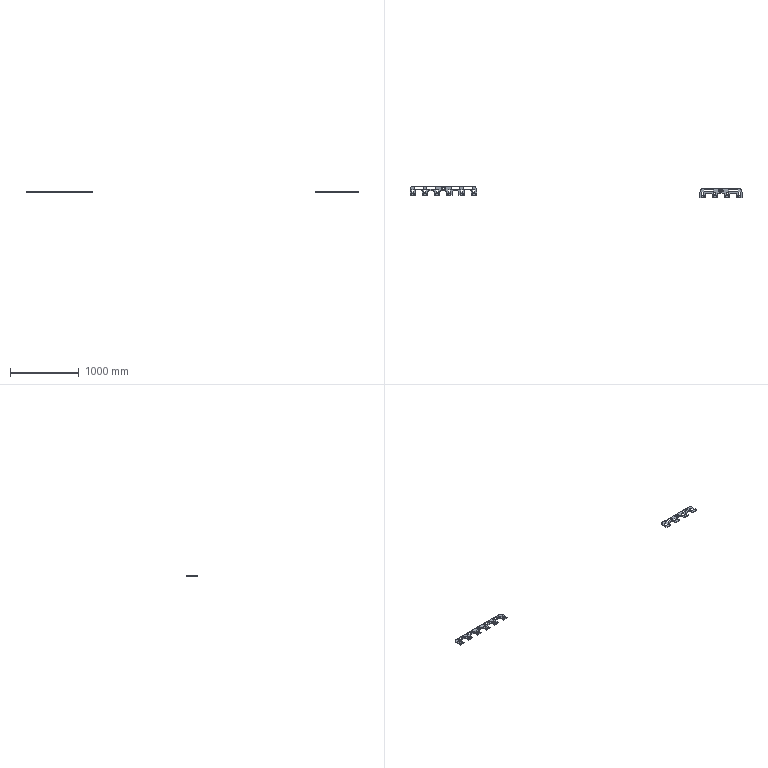NC program | NX | posted with a generic post | part box 4825 x 168.213 x 13 mm
Lines 1 to 137 of 14244:
N10 G17 G21 G94 G90
(FLOOR_WALL_COPY , TOOL : D63)
N12 T01 M6
N14 G54
N16 G17 G0 G90 X-36.5 Y68.997 S6500 M3
N18 G43 Z30. H1
N20 Z4.
N22 G94 G1 Z1. F1500.
N24 X-33.5
N26 X1000.3
N28 Y40.798
N30 X-33.5
N32 Y12.599
N34 X1000.3
N36 Y-15.601
N38 X-33.5
N40 Y-43.8
N42 X1000.3
N44 X1003.3
N46 Z4.
N48 G0 Z30.
N50 X-36.5 Y68.997
N52 Z3.
N54 G1 Z0.
N56 X-33.5
N58 X1000.3
N60 Y40.798
N62 X-33.5
N64 Y12.599
N66 X1000.3
N68 Y-15.601
N70 X-33.5
N72 Y-43.8
N74 X1000.3
N76 X1003.3
N78 Z3.
N80 G0 Z30.
N82 M5
(DRILLING_COPY_1 , TOOL : D6A45)
N84 T07 M6
N86 G54
N88 G17 G0 G90 X947.9 Y-61.2 S5000 M3
N90 G43 Z30. H7
N92 G94 G81 G98 Z-1. F250. R3.
N94 Y-39.2
N96 X907.9
N98 Y-61.2
N100 X770.1 Y-39.2
N102 Y-61.2
N104 X730.1
N106 Y-39.2
N108 X592.3
N110 Y-61.2
N112 X552.3
N114 Y-39.2
N116 X494.115 Y7.131
N118 X509.269 Y22.285
N120 Y43.715
N122 X494.115 Y58.869
N124 X472.685
N126 X457.531 Y43.715
N128 Y22.285
N130 X483.4 Y33.
N132 X472.685 Y7.131
N134 X414.5 Y-39.2
N136 Y-61.2
N138 X374.5
N140 Y-39.2
N142 X236.7
N144 Y-61.2
N146 X196.7
N148 Y-39.2
N150 X58.9
N152 Y-61.2
N154 X18.9
N156 Y-39.2
N158 G80
N160 G0 X18.9 Y-39.2 Z30.
N162 M5
(DRILLING_COPY_COPY_1 , TOOL : 4.5ZT)
N164 T14 M6
N166 G54
N168 G17 G0 G90 X457.531 Y43.715 S2000 M3
N170 G43 Z30. H14
N172 G94 G83 G98 Z-15.352 F250. Q2. R3.
N174 X472.685 Y58.869
N176 X494.115
N178 X509.269 Y43.715
N180 Y22.285
N182 X494.115 Y7.131
N184 X472.685
N186 X457.531 Y22.285
N188 G80
N190 G0 X457.531 Y22.285 Z30.
N192 M5
(DRILLING_COPY_COPY_COPY , TOOL : 6.5ZT)
N194 T15 M6
N196 G54
N198 G17 G0 G90 X947.9 Y-39.2 S2000 M3
N200 G43 Z30. H15
N202 G94 G83 G98 Z-15.953 F250. Q2. R3.
N204 Y-61.2
N206 X907.9
N208 Y-39.2
N210 X770.1
N212 Y-61.2
N214 X730.1
N216 Y-39.2
N218 X592.3 Y-61.2
N220 Y-39.2
N222 X552.3
N224 Y-61.2
N226 X414.5
N228 Y-39.2
N230 X374.5
N232 Y-61.2
N234 X236.7
N236 Y-39.2
N238 X196.7
N240 Y-61.2
N242 X58.9
N244 Y-39.2
N246 X18.9
N248 Y-61.2
N250 G80
N252 G0 X18.9 Y-61.2 Z30.
N254 M5